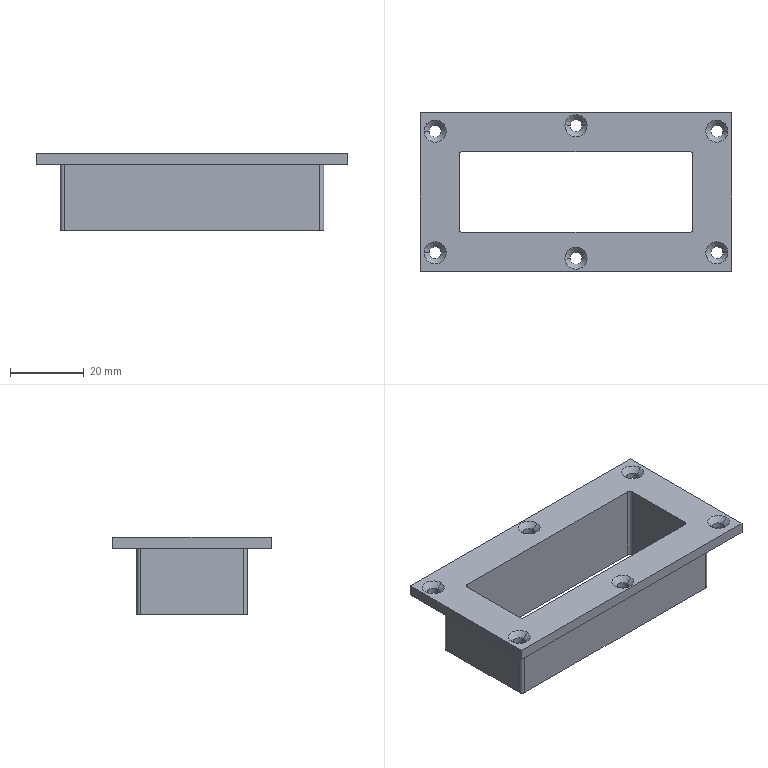Part | SolidWorks | features ICE 3, Fillet 2, Extrusion 1, HoleWzd 1 | 1 solid | 65 faces | box 84.5 x 43 x 21 mm | volume 19535 mm3 | cylinder 28 | plane 25 | cone 12 | commonest cylinder face diameters 2 x16 3.2 x12